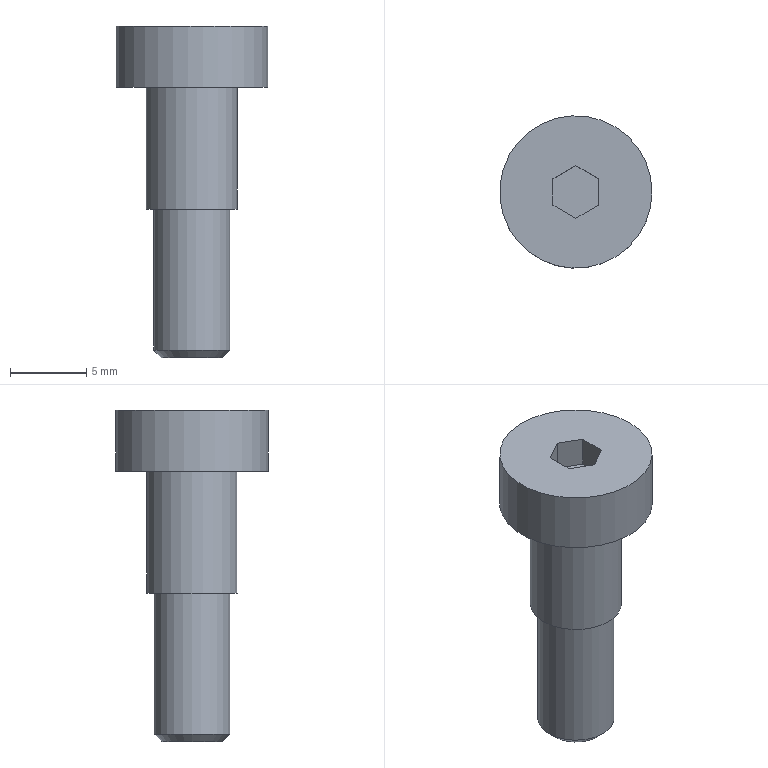Part | NX | features BREP 1, DATUM_CSYS 1 | 1 solid | 15 faces | box 10 x 10 x 21.75 mm | volume 714.374 mm3 | plane 11 | cylinder 3 | cone 1 | commonest cylinder face diameters 5 x1 6 x1 10 x1
STEP:
#1=CARTESIAN_POINT('',(1.5,0.866,2.));
#2=VERTEX_POINT('',#1);
#3=CARTESIAN_POINT('',(0.,1.732,2.));
#4=VERTEX_POINT('',#3);
#5=CARTESIAN_POINT('',(1.5,0.866,2.));
#6=DIRECTION('',(-0.866,0.5,0.));
#7=VECTOR('',#6,1000.);
#8=LINE('',#5,#7);
#9=EDGE_CURVE('',#2,#4,#8,.T.);
#10=ORIENTED_EDGE('',*,*,#9,.T.);
#11=CARTESIAN_POINT('',(-1.5,0.866,2.));
#12=VERTEX_POINT('',#11);
#13=CARTESIAN_POINT('',(0.,1.732,2.));
#14=DIRECTION('',(-0.866,-0.5,0.));
#15=VECTOR('',#14,1000.);
#16=LINE('',#13,#15);
#17=EDGE_CURVE('',#4,#12,#16,.T.);
#18=ORIENTED_EDGE('',*,*,#17,.T.);
#19=CARTESIAN_POINT('',(-1.5,-0.866,2.));
#20=VERTEX_POINT('',#19);
#21=CARTESIAN_POINT('',(-1.5,0.866,2.));
#22=DIRECTION('',(0.,-1.,0.));
#23=VECTOR('',#22,1000.);
#24=LINE('',#21,#23);
#25=EDGE_CURVE('',#12,#20,#24,.T.);
#26=ORIENTED_EDGE('',*,*,#25,.T.);
#27=CARTESIAN_POINT('',(0.,-1.732,2.));
#28=VERTEX_POINT('',#27);
#29=CARTESIAN_POINT('',(-1.5,-0.866,2.));
#30=DIRECTION('',(0.866,-0.5,0.));
#31=VECTOR('',#30,1000.);
#32=LINE('',#29,#31);
#33=EDGE_CURVE('',#20,#28,#32,.T.);
#34=ORIENTED_EDGE('',*,*,#33,.T.);
#35=CARTESIAN_POINT('',(1.5,-0.866,2.));
#36=VERTEX_POINT('',#35);
#37=CARTESIAN_POINT('',(0.,-1.732,2.));
#38=DIRECTION('',(0.866,0.5,0.));
#39=VECTOR('',#38,1000.);
#40=LINE('',#37,#39);
#41=EDGE_CURVE('',#28,#36,#40,.T.);
#42=ORIENTED_EDGE('',*,*,#41,.T.);
#43=CARTESIAN_POINT('',(1.5,-0.866,2.));
#44=DIRECTION('',(0.,1.,0.));
#45=VECTOR('',#44,1000.);
#46=LINE('',#43,#45);
#47=EDGE_CURVE('',#36,#2,#46,.T.);
#48=ORIENTED_EDGE('',*,*,#47,.T.);
#49=EDGE_LOOP('',(#10,#18,#26,#34,#42,#48));
#50=FACE_BOUND('',#49,.T.);
#51=CARTESIAN_POINT('',(0.2321,0.,2.));
#52=DIRECTION('',(0.,0.,1.));
#53=DIRECTION('',(-1.,0.,0.));
#54=AXIS2_PLACEMENT_3D('',#51,#52,#53);
#55=PLANE('',#54);
#56=ADVANCED_FACE('',(#50),#55,.T.);
#57=CARTESIAN_POINT('',(1.5,0.866,4.));
#58=VERTEX_POINT('',#57);
#59=CARTESIAN_POINT('',(0.,1.732,4.));
#60=VERTEX_POINT('',#59);
#61=CARTESIAN_POINT('',(1.5,0.866,4.));
#62=DIRECTION('',(-0.866,0.5,0.));
#63=VECTOR('',#62,1000.);
#64=LINE('',#61,#63);
#65=EDGE_CURVE('',#58,#60,#64,.T.);
#66=ORIENTED_EDGE('',*,*,#65,.T.);
#67=CARTESIAN_POINT('',(0.,1.732,4.));
#68=DIRECTION('',(0.,0.,-1.));
#69=VECTOR('',#68,1000.);
#70=LINE('',#67,#69);
#71=EDGE_CURVE('',#60,#4,#70,.T.);
#72=ORIENTED_EDGE('',*,*,#71,.T.);
#73=ORIENTED_EDGE('',*,*,#9,.F.);
#74=CARTESIAN_POINT('',(1.5,0.866,4.));
#75=DIRECTION('',(0.,0.,-1.));
#76=VECTOR('',#75,1000.);
#77=LINE('',#74,#76);
#78=EDGE_CURVE('',#58,#2,#77,.T.);
#79=ORIENTED_EDGE('',*,*,#78,.F.);
#80=EDGE_LOOP('',(#66,#72,#73,#79));
#81=FACE_BOUND('',#80,.T.);
#82=CARTESIAN_POINT('',(0.75,1.299,3.));
#83=DIRECTION('',(-0.5,-0.866,0.));
#84=DIRECTION('',(0.866,-0.5,0.));
#85=AXIS2_PLACEMENT_3D('',#82,#83,#84);
#86=PLANE('',#85);
#87=ADVANCED_FACE('',(#81),#86,.T.);
#88=CARTESIAN_POINT('',(-1.5,0.866,4.));
#89=VERTEX_POINT('',#88);
#90=CARTESIAN_POINT('',(0.,1.732,4.));
#91=DIRECTION('',(-0.866,-0.5,0.));
#92=VECTOR('',#91,1000.);
#93=LINE('',#90,#92);
#94=EDGE_CURVE('',#60,#89,#93,.T.);
#95=ORIENTED_EDGE('',*,*,#94,.T.);
#96=CARTESIAN_POINT('',(-1.5,0.866,4.));
#97=DIRECTION('',(0.,0.,-1.));
#98=VECTOR('',#97,1000.);
#99=LINE('',#96,#98);
#100=EDGE_CURVE('',#89,#12,#99,.T.);
#101=ORIENTED_EDGE('',*,*,#100,.T.);
#102=ORIENTED_EDGE('',*,*,#17,.F.);
#103=ORIENTED_EDGE('',*,*,#71,.F.);
#104=EDGE_LOOP('',(#95,#101,#102,#103));
#105=FACE_BOUND('',#104,.T.);
#106=CARTESIAN_POINT('',(-0.75,1.299,3.));
#107=DIRECTION('',(0.5,-0.866,0.));
#108=DIRECTION('',(0.866,0.5,0.));
#109=AXIS2_PLACEMENT_3D('',#106,#107,#108);
#110=PLANE('',#109);
#111=ADVANCED_FACE('',(#105),#110,.T.);
#112=CARTESIAN_POINT('',(-1.5,-0.866,4.));
#113=VERTEX_POINT('',#112);
#114=CARTESIAN_POINT('',(-1.5,0.866,4.));
#115=DIRECTION('',(0.,-1.,0.));
#116=VECTOR('',#115,1000.);
#117=LINE('',#114,#116);
#118=EDGE_CURVE('',#89,#113,#117,.T.);
#119=ORIENTED_EDGE('',*,*,#118,.T.);
#120=CARTESIAN_POINT('',(-1.5,-0.866,4.));
#121=DIRECTION('',(0.,0.,-1.));
#122=VECTOR('',#121,1000.);
#123=LINE('',#120,#122);
#124=EDGE_CURVE('',#113,#20,#123,.T.);
#125=ORIENTED_EDGE('',*,*,#124,.T.);
#126=ORIENTED_EDGE('',*,*,#25,.F.);
#127=ORIENTED_EDGE('',*,*,#100,.F.);
#128=EDGE_LOOP('',(#119,#125,#126,#127));
#129=FACE_BOUND('',#128,.T.);
#130=CARTESIAN_POINT('',(-1.5,0.,3.));
#131=DIRECTION('',(1.,0.,0.));
#132=DIRECTION('',(0.,1.,0.));
#133=AXIS2_PLACEMENT_3D('',#130,#131,#132);
#134=PLANE('',#133);
#135=ADVANCED_FACE('',(#129),#134,.T.);
#136=CARTESIAN_POINT('',(0.,-1.732,4.));
#137=VERTEX_POINT('',#136);
#138=CARTESIAN_POINT('',(-1.5,-0.866,4.));
#139=DIRECTION('',(0.866,-0.5,0.));
#140=VECTOR('',#139,1000.);
#141=LINE('',#138,#140);
#142=EDGE_CURVE('',#113,#137,#141,.T.);
#143=ORIENTED_EDGE('',*,*,#142,.T.);
#144=CARTESIAN_POINT('',(0.,-1.732,4.));
#145=DIRECTION('',(0.,0.,-1.));
#146=VECTOR('',#145,1000.);
#147=LINE('',#144,#146);
#148=EDGE_CURVE('',#137,#28,#147,.T.);
#149=ORIENTED_EDGE('',*,*,#148,.T.);
#150=ORIENTED_EDGE('',*,*,#33,.F.);
#151=ORIENTED_EDGE('',*,*,#124,.F.);
#152=EDGE_LOOP('',(#143,#149,#150,#151));
#153=FACE_BOUND('',#152,.T.);
#154=CARTESIAN_POINT('',(-0.75,-1.299,3.));
#155=DIRECTION('',(0.5,0.866,0.));
#156=DIRECTION('',(-0.866,0.5,0.));
#157=AXIS2_PLACEMENT_3D('',#154,#155,#156);
#158=PLANE('',#157);
#159=ADVANCED_FACE('',(#153),#158,.T.);
#160=CARTESIAN_POINT('',(1.5,-0.866,4.));
#161=VERTEX_POINT('',#160);
#162=CARTESIAN_POINT('',(0.,-1.732,4.));
#163=DIRECTION('',(0.866,0.5,0.));
#164=VECTOR('',#163,1000.);
#165=LINE('',#162,#164);
#166=EDGE_CURVE('',#137,#161,#165,.T.);
#167=ORIENTED_EDGE('',*,*,#166,.T.);
#168=CARTESIAN_POINT('',(1.5,-0.866,4.));
#169=DIRECTION('',(0.,0.,-1.));
#170=VECTOR('',#169,1000.);
#171=LINE('',#168,#170);
#172=EDGE_CURVE('',#161,#36,#171,.T.);
#173=ORIENTED_EDGE('',*,*,#172,.T.);
#174=ORIENTED_EDGE('',*,*,#41,.F.);
#175=ORIENTED_EDGE('',*,*,#148,.F.);
#176=EDGE_LOOP('',(#167,#173,#174,#175));
#177=FACE_BOUND('',#176,.T.);
#178=CARTESIAN_POINT('',(0.75,-1.299,3.));
#179=DIRECTION('',(-0.5,0.866,0.));
#180=DIRECTION('',(-0.866,-0.5,0.));
#181=AXIS2_PLACEMENT_3D('',#178,#179,#180);
#182=PLANE('',#181);
#183=ADVANCED_FACE('',(#177),#182,.T.);
#184=CARTESIAN_POINT('',(1.5,-0.866,4.));
#185=DIRECTION('',(0.,1.,0.));
#186=VECTOR('',#185,1000.);
#187=LINE('',#184,#186);
#188=EDGE_CURVE('',#161,#58,#187,.T.);
#189=ORIENTED_EDGE('',*,*,#188,.T.);
#190=ORIENTED_EDGE('',*,*,#78,.T.);
#191=ORIENTED_EDGE('',*,*,#47,.F.);
#192=ORIENTED_EDGE('',*,*,#172,.F.);
#193=EDGE_LOOP('',(#189,#190,#191,#192));
#194=FACE_BOUND('',#193,.T.);
#195=CARTESIAN_POINT('',(1.5,0.,3.));
#196=DIRECTION('',(-1.,0.,0.));
#197=DIRECTION('',(0.,-1.,0.));
#198=AXIS2_PLACEMENT_3D('',#195,#196,#197);
#199=PLANE('',#198);
#200=ADVANCED_FACE('',(#194),#199,.T.);
#201=CARTESIAN_POINT('',(5.,0.,4.));
#202=VERTEX_POINT('',#201);
#203=CARTESIAN_POINT('',(0.,0.,4.));
#204=DIRECTION('',(0.,0.,1.));
#205=DIRECTION('',(1.,0.,0.));
#206=AXIS2_PLACEMENT_3D('',#203,#204,#205);
#207=CIRCLE('',#206,5.);
#208=EDGE_CURVE('',#202,#202,#207,.T.);
#209=ORIENTED_EDGE('',*,*,#208,.T.);
#210=EDGE_LOOP('',(#209));
#211=FACE_BOUND('',#210,.T.);
#212=ORIENTED_EDGE('',*,*,#94,.F.);
#213=ORIENTED_EDGE('',*,*,#65,.F.);
#214=ORIENTED_EDGE('',*,*,#188,.F.);
#215=ORIENTED_EDGE('',*,*,#166,.F.);
#216=ORIENTED_EDGE('',*,*,#142,.F.);
#217=ORIENTED_EDGE('',*,*,#118,.F.);
#218=EDGE_LOOP('',(#212,#213,#214,#215,#216,#217));
#219=FACE_BOUND('',#218,.T.);
#220=CARTESIAN_POINT('',(0.,0.,4.));
#221=DIRECTION('',(0.,0.,1.));
#222=DIRECTION('',(-1.,0.,0.));
#223=AXIS2_PLACEMENT_3D('',#220,#221,#222);
#224=PLANE('',#223);
#225=ADVANCED_FACE('',(#211,#219),#224,.T.);
#226=CARTESIAN_POINT('',(5.,0.,0.));
#227=VERTEX_POINT('',#226);
#228=CARTESIAN_POINT('',(0.,0.,0.));
#229=DIRECTION('',(0.,0.,1.));
#230=DIRECTION('',(1.,0.,0.));
#231=AXIS2_PLACEMENT_3D('',#228,#229,#230);
#232=CIRCLE('',#231,5.);
#233=EDGE_CURVE('',#227,#227,#232,.T.);
#234=ORIENTED_EDGE('',*,*,#233,.T.);
#235=CARTESIAN_POINT('',(5.,0.,0.));
#236=DIRECTION('',(0.,0.,1.));
#237=VECTOR('',#236,1000.);
#238=LINE('',#235,#237);
#239=EDGE_CURVE('',#227,#202,#238,.T.);
#240=ORIENTED_EDGE('',*,*,#239,.T.);
#241=ORIENTED_EDGE('',*,*,#208,.F.);
#242=ORIENTED_EDGE('',*,*,#239,.F.);
#243=EDGE_LOOP('',(#234,#240,#241,#242));
#244=FACE_BOUND('',#243,.T.);
#245=CARTESIAN_POINT('',(0.,0.,0.));
#246=DIRECTION('',(0.,0.,1.));
#247=DIRECTION('',(-1.,0.,0.));
#248=AXIS2_PLACEMENT_3D('',#245,#246,#247);
#249=CYLINDRICAL_SURFACE('',#248,5.);
#250=ADVANCED_FACE('',(#244),#249,.T.);
#251=ORIENTED_EDGE('',*,*,#233,.F.);
#252=EDGE_LOOP('',(#251));
#253=FACE_BOUND('',#252,.T.);
#254=CARTESIAN_POINT('',(3.,0.,0.));
#255=VERTEX_POINT('',#254);
#256=CARTESIAN_POINT('',(0.,0.,0.));
#257=DIRECTION('',(0.,0.,-1.));
#258=DIRECTION('',(1.,0.,0.));
#259=AXIS2_PLACEMENT_3D('',#256,#257,#258);
#260=CIRCLE('',#259,3.);
#261=EDGE_CURVE('',#255,#255,#260,.T.);
#262=ORIENTED_EDGE('',*,*,#261,.F.);
#263=EDGE_LOOP('',(#262));
#264=FACE_BOUND('',#263,.T.);
#265=CARTESIAN_POINT('',(0.,0.,0.));
#266=DIRECTION('',(0.,0.,1.));
#267=DIRECTION('',(-1.,0.,0.));
#268=AXIS2_PLACEMENT_3D('',#265,#266,#267);
#269=PLANE('',#268);
#270=ADVANCED_FACE('',(#253,#264),#269,.F.);
#271=ORIENTED_EDGE('',*,*,#261,.T.);
#272=CARTESIAN_POINT('',(3.,0.,-8.));
#273=VERTEX_POINT('',#272);
#274=CARTESIAN_POINT('',(3.,0.,0.));
#275=DIRECTION('',(0.,0.,-1.));
#276=VECTOR('',#275,1000.);
#277=LINE('',#274,#276);
#278=EDGE_CURVE('',#255,#273,#277,.T.);
#279=ORIENTED_EDGE('',*,*,#278,.T.);
#280=CARTESIAN_POINT('',(0.,0.,-8.));
#281=DIRECTION('',(0.,0.,-1.));
#282=DIRECTION('',(1.,0.,0.));
#283=AXIS2_PLACEMENT_3D('',#280,#281,#282);
#284=CIRCLE('',#283,3.);
#285=EDGE_CURVE('',#273,#273,#284,.T.);
#286=ORIENTED_EDGE('',*,*,#285,.F.);
#287=ORIENTED_EDGE('',*,*,#278,.F.);
#288=EDGE_LOOP('',(#271,#279,#286,#287));
#289=FACE_BOUND('',#288,.T.);
#290=CARTESIAN_POINT('',(0.,0.,0.));
#291=DIRECTION('',(0.,0.,-1.));
#292=DIRECTION('',(-1.,0.,0.));
#293=AXIS2_PLACEMENT_3D('',#290,#291,#292);
#294=CYLINDRICAL_SURFACE('',#293,3.);
#295=ADVANCED_FACE('',(#289),#294,.T.);
#296=ORIENTED_EDGE('',*,*,#285,.T.);
#297=EDGE_LOOP('',(#296));
#298=FACE_BOUND('',#297,.T.);
#299=CARTESIAN_POINT('',(2.5,0.,-8.));
#300=VERTEX_POINT('',#299);
#301=CARTESIAN_POINT('',(0.,0.,-8.));
#302=DIRECTION('',(0.,0.,-1.));
#303=DIRECTION('',(1.,0.,0.));
#304=AXIS2_PLACEMENT_3D('',#301,#302,#303);
#305=CIRCLE('',#304,2.5);
#306=EDGE_CURVE('',#300,#300,#305,.T.);
#307=ORIENTED_EDGE('',*,*,#306,.F.);
#308=EDGE_LOOP('',(#307));
#309=FACE_BOUND('',#308,.T.);
#310=CARTESIAN_POINT('',(0.,0.,-8.));
#311=DIRECTION('',(0.,0.,-1.));
#312=DIRECTION('',(-1.,0.,0.));
#313=AXIS2_PLACEMENT_3D('',#310,#311,#312);
#314=PLANE('',#313);
#315=ADVANCED_FACE('',(#298,#309),#314,.T.);
#316=ORIENTED_EDGE('',*,*,#306,.T.);
#317=CARTESIAN_POINT('',(2.5,0.,-17.25));
#318=VERTEX_POINT('',#317);
#319=CARTESIAN_POINT('',(2.5,0.,-8.));
#320=DIRECTION('',(0.,0.,-1.));
#321=VECTOR('',#320,1000.);
#322=LINE('',#319,#321);
#323=EDGE_CURVE('',#300,#318,#322,.T.);
#324=ORIENTED_EDGE('',*,*,#323,.T.);
#325=CARTESIAN_POINT('',(0.,0.,-17.25));
#326=DIRECTION('',(0.,0.,1.));
#327=DIRECTION('',(1.,0.,0.));
#328=AXIS2_PLACEMENT_3D('',#325,#326,#327);
#329=CIRCLE('',#328,2.5);
#330=EDGE_CURVE('',#318,#318,#329,.T.);
#331=ORIENTED_EDGE('',*,*,#330,.T.);
#332=ORIENTED_EDGE('',*,*,#323,.F.);
#333=EDGE_LOOP('',(#316,#324,#331,#332));
#334=FACE_BOUND('',#333,.T.);
#335=CARTESIAN_POINT('',(0.,0.,-8.));
#336=DIRECTION('',(0.,0.,-1.));
#337=DIRECTION('',(-1.,0.,0.));
#338=AXIS2_PLACEMENT_3D('',#335,#336,#337);
#339=CYLINDRICAL_SURFACE('',#338,2.5);
#340=ADVANCED_FACE('',(#334),#339,.T.);
#341=CARTESIAN_POINT('',(2.,0.,-17.75));
#342=VERTEX_POINT('',#341);
#343=CARTESIAN_POINT('',(0.,0.,-17.75));
#344=DIRECTION('',(0.,0.,1.));
#345=DIRECTION('',(1.,0.,0.));
#346=AXIS2_PLACEMENT_3D('',#343,#344,#345);
#347=CIRCLE('',#346,2.);
#348=EDGE_CURVE('',#342,#342,#347,.T.);
#349=ORIENTED_EDGE('',*,*,#348,.F.);
#350=EDGE_LOOP('',(#349));
#351=FACE_BOUND('',#350,.T.);
#352=CARTESIAN_POINT('',(0.,0.,-17.75));
#353=DIRECTION('',(0.,0.,-1.));
#354=DIRECTION('',(-1.,0.,0.));
#355=AXIS2_PLACEMENT_3D('',#352,#353,#354);
#356=PLANE('',#355);
#357=ADVANCED_FACE('',(#351),#356,.T.);
#358=CARTESIAN_POINT('',(2.,0.,-17.75));
#359=DIRECTION('',(0.7071,0.,0.7071));
#360=VECTOR('',#359,1000.);
#361=LINE('',#358,#360);
#362=EDGE_CURVE('',#342,#318,#361,.T.);
#363=ORIENTED_EDGE('',*,*,#362,.T.);
#364=ORIENTED_EDGE('',*,*,#330,.F.);
#365=ORIENTED_EDGE('',*,*,#362,.F.);
#366=ORIENTED_EDGE('',*,*,#348,.T.);
#367=EDGE_LOOP('',(#363,#364,#365,#366));
#368=FACE_BOUND('',#367,.T.);
#369=CARTESIAN_POINT('',(0.,0.,-17.75));
#370=DIRECTION('',(0.,0.,1.));
#371=DIRECTION('',(-1.,0.,0.));
#372=AXIS2_PLACEMENT_3D('',#369,#370,#371);
#373=CONICAL_SURFACE('',#372,2.,0.7854);
#374=ADVANCED_FACE('',(#368),#373,.T.);
#375=CLOSED_SHELL('',(#56,#87,#111,#135,#159,#183,#200,#225,#250,#270,#295,#315,#340,#357,#374));
#376=MANIFOLD_SOLID_BREP('',#375);
#377=(LENGTH_UNIT()NAMED_UNIT(*)SI_UNIT(.MILLI.,.METRE.));
#378=UNCERTAINTY_MEASURE_WITH_UNIT(LENGTH_MEASURE(0.00001),#377,'','');
#379=(NAMED_UNIT(*)PLANE_ANGLE_UNIT()SI_UNIT($,.RADIAN.));
#380=(NAMED_UNIT(*)SI_UNIT($,.STERADIAN.)SOLID_ANGLE_UNIT());
#381=(GEOMETRIC_REPRESENTATION_CONTEXT(3)GLOBAL_UNCERTAINTY_ASSIGNED_CONTEXT((#378))GLOBAL_UNIT_ASSIGNED_CONTEXT((#377,#379,#380))REPRESENTATION_CONTEXT('',''));
#382=ADVANCED_BREP_SHAPE_REPRESENTATION('',(#376),#381);